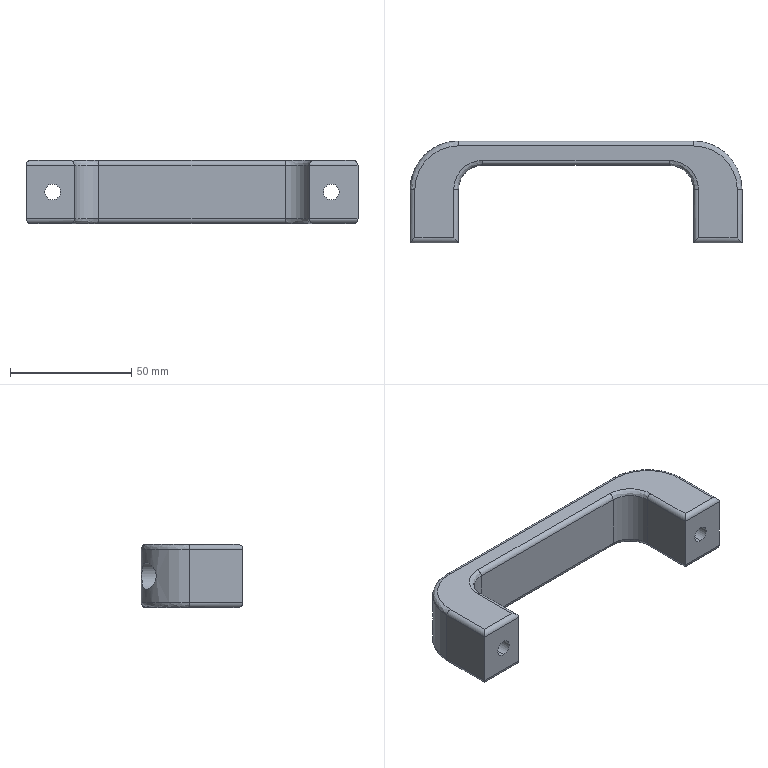Part | STEP file | Handle | 1 solid | 48 faces | box 137 x 42 x 26 mm | volume 58032 mm3 | cylinder 28 | plane 12 | spline 8 | commonest cylinder face diameters 4 x16 6.6 x4 11 x4 20 x2 40 x2